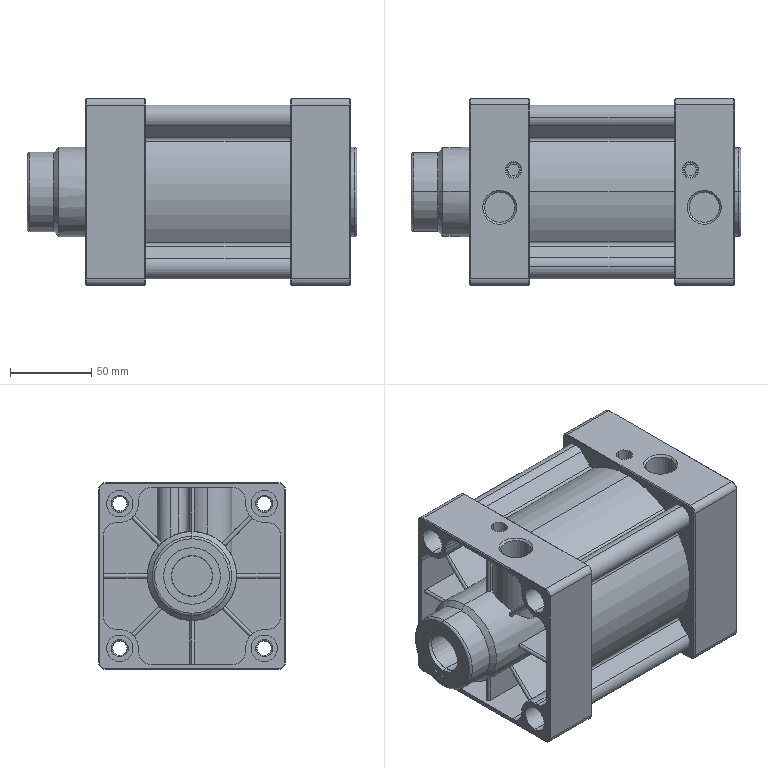Part | STEP file | 1 solid | 354 faces | box 203 x 115 x 115 mm | volume 819045 mm3 | cylinder 158 | plane 146 | cone 46 | torus 4 | commonest cylinder face diameters 16 x21 2.7 x18 10.7 x16 16.3 x16 8 x11 4 x10